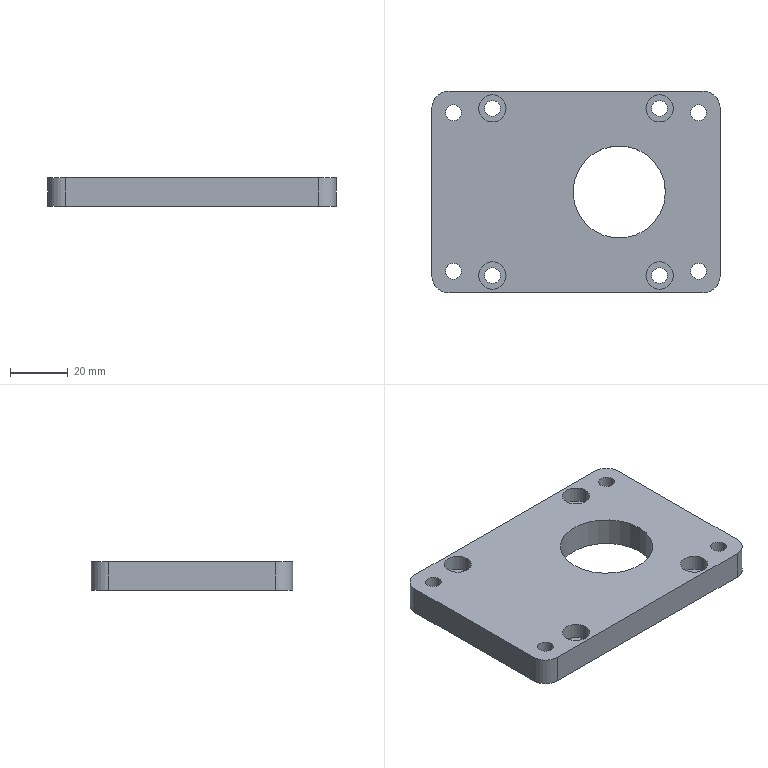Part | STEP file | QA-FC08 | 1 solid | 52 faces | box 100 x 70 x 10 mm | volume 57674 mm3 | cylinder 38 | plane 14 | commonest cylinder face diameters 5.5 x16 9.5 x16 12 x4 32 x2